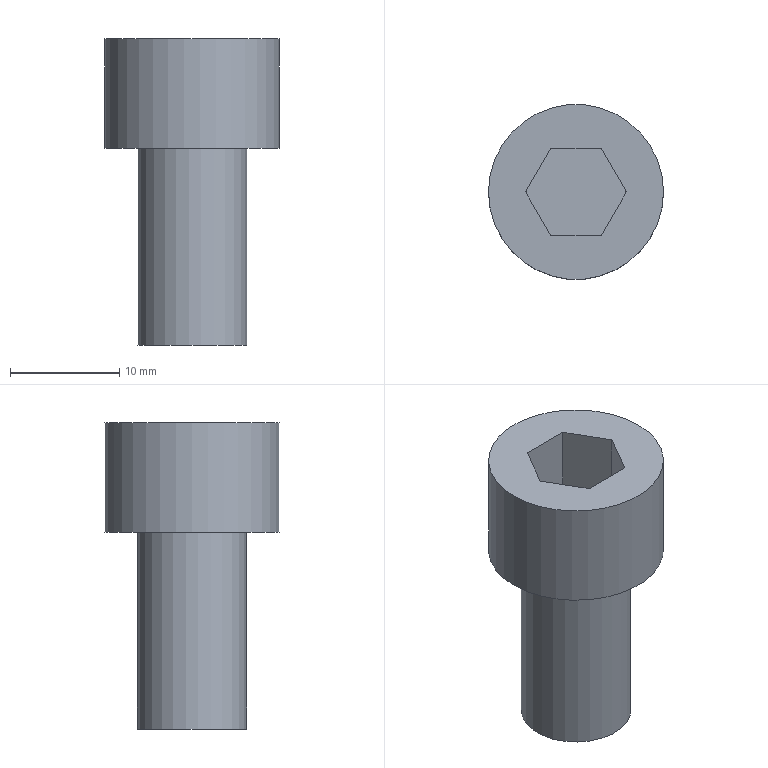Part | STEP file | 冲床-300配套压波_id138_x_t | 1 solid | 12 faces | box 16 x 16 x 28 mm | volume 3059 mm3 | plane 10 | cylinder 2 | commonest cylinder face diameters 10 x1 16 x1
STEP:
#1=CARTESIAN_POINT('',(1204.,86.,299.));
#2=VERTEX_POINT('',#1);
#3=CARTESIAN_POINT('',(1196.,86.,299.));
#4=DIRECTION('',(0.,0.,1.));
#5=DIRECTION('',(1.,0.,0.));
#6=AXIS2_PLACEMENT_3D('',#3,#4,#5);
#7=CIRCLE('',#6,8.);
#8=EDGE_CURVE('',#2,#2,#7,.T.);
#9=ORIENTED_EDGE('',*,*,#8,.T.);
#10=EDGE_LOOP('',(#9));
#11=FACE_BOUND('',#10,.T.);
#12=CARTESIAN_POINT('',(1193.691,90.,299.));
#13=VERTEX_POINT('',#12);
#14=CARTESIAN_POINT('',(1198.309,90.,299.));
#15=VERTEX_POINT('',#14);
#16=CARTESIAN_POINT('',(1193.691,90.,299.));
#17=DIRECTION('',(1.,0.,0.));
#18=VECTOR('',#17,1.);
#19=LINE('',#16,#18);
#20=EDGE_CURVE('',#13,#15,#19,.T.);
#21=ORIENTED_EDGE('',*,*,#20,.T.);
#22=CARTESIAN_POINT('',(1200.619,86.,299.));
#23=VERTEX_POINT('',#22);
#24=CARTESIAN_POINT('',(1198.309,90.,299.));
#25=DIRECTION('',(0.5,-0.866,0.));
#26=VECTOR('',#25,1.);
#27=LINE('',#24,#26);
#28=EDGE_CURVE('',#15,#23,#27,.T.);
#29=ORIENTED_EDGE('',*,*,#28,.T.);
#30=CARTESIAN_POINT('',(1198.309,82.,299.));
#31=VERTEX_POINT('',#30);
#32=CARTESIAN_POINT('',(1200.619,86.,299.));
#33=DIRECTION('',(-0.5,-0.866,0.));
#34=VECTOR('',#33,1.);
#35=LINE('',#32,#34);
#36=EDGE_CURVE('',#23,#31,#35,.T.);
#37=ORIENTED_EDGE('',*,*,#36,.T.);
#38=CARTESIAN_POINT('',(1193.691,82.,299.));
#39=VERTEX_POINT('',#38);
#40=CARTESIAN_POINT('',(1198.309,82.,299.));
#41=DIRECTION('',(-1.,0.,0.));
#42=VECTOR('',#41,1.);
#43=LINE('',#40,#42);
#44=EDGE_CURVE('',#31,#39,#43,.T.);
#45=ORIENTED_EDGE('',*,*,#44,.T.);
#46=CARTESIAN_POINT('',(1191.381,86.,299.));
#47=VERTEX_POINT('',#46);
#48=CARTESIAN_POINT('',(1193.691,82.,299.));
#49=DIRECTION('',(-0.5,0.866,0.));
#50=VECTOR('',#49,1.);
#51=LINE('',#48,#50);
#52=EDGE_CURVE('',#39,#47,#51,.T.);
#53=ORIENTED_EDGE('',*,*,#52,.T.);
#54=CARTESIAN_POINT('',(1191.381,86.,299.));
#55=DIRECTION('',(0.5,0.866,0.));
#56=VECTOR('',#55,1.);
#57=LINE('',#54,#56);
#58=EDGE_CURVE('',#47,#13,#57,.T.);
#59=ORIENTED_EDGE('',*,*,#58,.T.);
#60=EDGE_LOOP('',(#21,#29,#37,#45,#53,#59));
#61=FACE_BOUND('',#60,.T.);
#62=CARTESIAN_POINT('',(1204.,86.,299.));
#63=DIRECTION('',(0.,0.,-1.));
#64=DIRECTION('',(-1.,0.,0.));
#65=AXIS2_PLACEMENT_3D('',#62,#63,#64);
#66=PLANE('',#65);
#67=ADVANCED_FACE('',(#11,#61),#66,.F.);
#68=ORIENTED_EDGE('',*,*,#8,.F.);
#69=EDGE_LOOP('',(#68));
#70=FACE_BOUND('',#69,.T.);
#71=CARTESIAN_POINT('',(1204.,86.,289.));
#72=VERTEX_POINT('',#71);
#73=CARTESIAN_POINT('',(1196.,86.,289.));
#74=DIRECTION('',(0.,0.,1.));
#75=DIRECTION('',(1.,0.,0.));
#76=AXIS2_PLACEMENT_3D('',#73,#74,#75);
#77=CIRCLE('',#76,8.);
#78=EDGE_CURVE('',#72,#72,#77,.T.);
#79=ORIENTED_EDGE('',*,*,#78,.T.);
#80=EDGE_LOOP('',(#79));
#81=FACE_BOUND('',#80,.T.);
#82=CARTESIAN_POINT('',(1196.,86.,290.1));
#83=DIRECTION('',(0.,0.,1.));
#84=DIRECTION('',(1.,0.,0.));
#85=AXIS2_PLACEMENT_3D('',#82,#83,#84);
#86=CYLINDRICAL_SURFACE('',#85,8.);
#87=ADVANCED_FACE('',(#70,#81),#86,.T.);
#88=ORIENTED_EDGE('',*,*,#78,.F.);
#89=EDGE_LOOP('',(#88));
#90=FACE_BOUND('',#89,.T.);
#91=CARTESIAN_POINT('',(1201.,86.,289.));
#92=VERTEX_POINT('',#91);
#93=CARTESIAN_POINT('',(1196.,86.,289.));
#94=DIRECTION('',(0.,0.,1.));
#95=DIRECTION('',(1.,0.,0.));
#96=AXIS2_PLACEMENT_3D('',#93,#94,#95);
#97=CIRCLE('',#96,5.);
#98=EDGE_CURVE('',#92,#92,#97,.T.);
#99=ORIENTED_EDGE('',*,*,#98,.T.);
#100=EDGE_LOOP('',(#99));
#101=FACE_BOUND('',#100,.T.);
#102=CARTESIAN_POINT('',(1201.,86.,289.));
#103=DIRECTION('',(0.,0.,1.));
#104=DIRECTION('',(1.,0.,0.));
#105=AXIS2_PLACEMENT_3D('',#102,#103,#104);
#106=PLANE('',#105);
#107=ADVANCED_FACE('',(#90,#101),#106,.F.);
#108=ORIENTED_EDGE('',*,*,#98,.F.);
#109=EDGE_LOOP('',(#108));
#110=FACE_BOUND('',#109,.T.);
#111=CARTESIAN_POINT('',(1201.,86.,271.));
#112=VERTEX_POINT('',#111);
#113=CARTESIAN_POINT('',(1196.,86.,271.));
#114=DIRECTION('',(0.,0.,1.));
#115=DIRECTION('',(1.,0.,0.));
#116=AXIS2_PLACEMENT_3D('',#113,#114,#115);
#117=CIRCLE('',#116,5.);
#118=EDGE_CURVE('',#112,#112,#117,.T.);
#119=ORIENTED_EDGE('',*,*,#118,.T.);
#120=EDGE_LOOP('',(#119));
#121=FACE_BOUND('',#120,.T.);
#122=CARTESIAN_POINT('',(1196.,86.,290.1));
#123=DIRECTION('',(0.,0.,1.));
#124=DIRECTION('',(1.,0.,0.));
#125=AXIS2_PLACEMENT_3D('',#122,#123,#124);
#126=CYLINDRICAL_SURFACE('',#125,5.);
#127=ADVANCED_FACE('',(#110,#121),#126,.T.);
#128=ORIENTED_EDGE('',*,*,#118,.F.);
#129=EDGE_LOOP('',(#128));
#130=FACE_OUTER_BOUND('',#129,.T.);
#131=CARTESIAN_POINT('',(1196.,86.,271.));
#132=DIRECTION('',(0.,0.,1.));
#133=DIRECTION('',(1.,0.,0.));
#134=AXIS2_PLACEMENT_3D('',#131,#132,#133);
#135=PLANE('',#134);
#136=ADVANCED_FACE('',(#130),#135,.F.);
#137=ORIENTED_EDGE('',*,*,#20,.F.);
#138=CARTESIAN_POINT('',(1193.691,90.,292.4));
#139=VERTEX_POINT('',#138);
#140=CARTESIAN_POINT('',(1193.691,90.,292.4));
#141=DIRECTION('',(0.,0.,-1.));
#142=VECTOR('',#141,1.);
#143=LINE('',#140,#142);
#144=EDGE_CURVE('',#13,#139,#143,.T.);
#145=ORIENTED_EDGE('',*,*,#144,.T.);
#146=CARTESIAN_POINT('',(1198.309,90.,292.4));
#147=VERTEX_POINT('',#146);
#148=CARTESIAN_POINT('',(1193.691,90.,292.4));
#149=DIRECTION('',(-1.,0.,0.));
#150=VECTOR('',#149,1.);
#151=LINE('',#148,#150);
#152=EDGE_CURVE('',#147,#139,#151,.T.);
#153=ORIENTED_EDGE('',*,*,#152,.F.);
#154=CARTESIAN_POINT('',(1198.309,90.,292.4));
#155=DIRECTION('',(0.,0.,-1.));
#156=VECTOR('',#155,1.);
#157=LINE('',#154,#156);
#158=EDGE_CURVE('',#15,#147,#157,.T.);
#159=ORIENTED_EDGE('',*,*,#158,.F.);
#160=EDGE_LOOP('',(#137,#145,#153,#159));
#161=FACE_OUTER_BOUND('',#160,.T.);
#162=CARTESIAN_POINT('',(1193.691,90.,292.4));
#163=DIRECTION('',(0.,-1.,0.));
#164=DIRECTION('',(1.,0.,0.));
#165=AXIS2_PLACEMENT_3D('',#162,#163,#164);
#166=PLANE('',#165);
#167=ADVANCED_FACE('',(#161),#166,.T.);
#168=ORIENTED_EDGE('',*,*,#28,.F.);
#169=ORIENTED_EDGE('',*,*,#158,.T.);
#170=CARTESIAN_POINT('',(1200.619,86.,292.4));
#171=VERTEX_POINT('',#170);
#172=CARTESIAN_POINT('',(1198.309,90.,292.4));
#173=DIRECTION('',(-0.5,0.866,0.));
#174=VECTOR('',#173,1.);
#175=LINE('',#172,#174);
#176=EDGE_CURVE('',#171,#147,#175,.T.);
#177=ORIENTED_EDGE('',*,*,#176,.F.);
#178=CARTESIAN_POINT('',(1200.619,86.,292.4));
#179=DIRECTION('',(0.,0.,-1.));
#180=VECTOR('',#179,1.);
#181=LINE('',#178,#180);
#182=EDGE_CURVE('',#23,#171,#181,.T.);
#183=ORIENTED_EDGE('',*,*,#182,.F.);
#184=EDGE_LOOP('',(#168,#169,#177,#183));
#185=FACE_OUTER_BOUND('',#184,.T.);
#186=CARTESIAN_POINT('',(1198.309,90.,292.4));
#187=DIRECTION('',(-0.866,-0.5,0.));
#188=DIRECTION('',(0.5,-0.866,0.));
#189=AXIS2_PLACEMENT_3D('',#186,#187,#188);
#190=PLANE('',#189);
#191=ADVANCED_FACE('',(#185),#190,.T.);
#192=ORIENTED_EDGE('',*,*,#36,.F.);
#193=ORIENTED_EDGE('',*,*,#182,.T.);
#194=CARTESIAN_POINT('',(1198.309,82.,292.4));
#195=VERTEX_POINT('',#194);
#196=CARTESIAN_POINT('',(1200.619,86.,292.4));
#197=DIRECTION('',(0.5,0.866,0.));
#198=VECTOR('',#197,1.);
#199=LINE('',#196,#198);
#200=EDGE_CURVE('',#195,#171,#199,.T.);
#201=ORIENTED_EDGE('',*,*,#200,.F.);
#202=CARTESIAN_POINT('',(1198.309,82.,292.4));
#203=DIRECTION('',(0.,0.,-1.));
#204=VECTOR('',#203,1.);
#205=LINE('',#202,#204);
#206=EDGE_CURVE('',#31,#195,#205,.T.);
#207=ORIENTED_EDGE('',*,*,#206,.F.);
#208=EDGE_LOOP('',(#192,#193,#201,#207));
#209=FACE_OUTER_BOUND('',#208,.T.);
#210=CARTESIAN_POINT('',(1200.619,86.,292.4));
#211=DIRECTION('',(-0.866,0.5,0.));
#212=DIRECTION('',(-0.5,-0.866,0.));
#213=AXIS2_PLACEMENT_3D('',#210,#211,#212);
#214=PLANE('',#213);
#215=ADVANCED_FACE('',(#209),#214,.T.);
#216=ORIENTED_EDGE('',*,*,#44,.F.);
#217=ORIENTED_EDGE('',*,*,#206,.T.);
#218=CARTESIAN_POINT('',(1193.691,82.,292.4));
#219=VERTEX_POINT('',#218);
#220=CARTESIAN_POINT('',(1198.309,82.,292.4));
#221=DIRECTION('',(1.,0.,0.));
#222=VECTOR('',#221,1.);
#223=LINE('',#220,#222);
#224=EDGE_CURVE('',#219,#195,#223,.T.);
#225=ORIENTED_EDGE('',*,*,#224,.F.);
#226=CARTESIAN_POINT('',(1193.691,82.,292.4));
#227=DIRECTION('',(0.,0.,-1.));
#228=VECTOR('',#227,1.);
#229=LINE('',#226,#228);
#230=EDGE_CURVE('',#39,#219,#229,.T.);
#231=ORIENTED_EDGE('',*,*,#230,.F.);
#232=EDGE_LOOP('',(#216,#217,#225,#231));
#233=FACE_OUTER_BOUND('',#232,.T.);
#234=CARTESIAN_POINT('',(1198.309,82.,292.4));
#235=DIRECTION('',(0.,1.,0.));
#236=DIRECTION('',(0.,0.,1.));
#237=AXIS2_PLACEMENT_3D('',#234,#235,#236);
#238=PLANE('',#237);
#239=ADVANCED_FACE('',(#233),#238,.T.);
#240=ORIENTED_EDGE('',*,*,#52,.F.);
#241=ORIENTED_EDGE('',*,*,#230,.T.);
#242=CARTESIAN_POINT('',(1191.381,86.,292.4));
#243=VERTEX_POINT('',#242);
#244=CARTESIAN_POINT('',(1193.691,82.,292.4));
#245=DIRECTION('',(0.5,-0.866,0.));
#246=VECTOR('',#245,1.);
#247=LINE('',#244,#246);
#248=EDGE_CURVE('',#243,#219,#247,.T.);
#249=ORIENTED_EDGE('',*,*,#248,.F.);
#250=CARTESIAN_POINT('',(1191.381,86.,292.4));
#251=DIRECTION('',(0.,0.,-1.));
#252=VECTOR('',#251,1.);
#253=LINE('',#250,#252);
#254=EDGE_CURVE('',#47,#243,#253,.T.);
#255=ORIENTED_EDGE('',*,*,#254,.F.);
#256=EDGE_LOOP('',(#240,#241,#249,#255));
#257=FACE_OUTER_BOUND('',#256,.T.);
#258=CARTESIAN_POINT('',(1193.691,82.,292.4));
#259=DIRECTION('',(0.866,0.5,0.));
#260=DIRECTION('',(-0.5,0.866,0.));
#261=AXIS2_PLACEMENT_3D('',#258,#259,#260);
#262=PLANE('',#261);
#263=ADVANCED_FACE('',(#257),#262,.T.);
#264=ORIENTED_EDGE('',*,*,#58,.F.);
#265=ORIENTED_EDGE('',*,*,#254,.T.);
#266=CARTESIAN_POINT('',(1191.381,86.,292.4));
#267=DIRECTION('',(-0.5,-0.866,0.));
#268=VECTOR('',#267,1.);
#269=LINE('',#266,#268);
#270=EDGE_CURVE('',#139,#243,#269,.T.);
#271=ORIENTED_EDGE('',*,*,#270,.F.);
#272=ORIENTED_EDGE('',*,*,#144,.F.);
#273=EDGE_LOOP('',(#264,#265,#271,#272));
#274=FACE_OUTER_BOUND('',#273,.T.);
#275=CARTESIAN_POINT('',(1191.381,86.,292.4));
#276=DIRECTION('',(0.866,-0.5,0.));
#277=DIRECTION('',(0.5,0.866,0.));
#278=AXIS2_PLACEMENT_3D('',#275,#276,#277);
#279=PLANE('',#278);
#280=ADVANCED_FACE('',(#274),#279,.T.);
#281=ORIENTED_EDGE('',*,*,#152,.T.);
#282=ORIENTED_EDGE('',*,*,#270,.T.);
#283=ORIENTED_EDGE('',*,*,#248,.T.);
#284=ORIENTED_EDGE('',*,*,#224,.T.);
#285=ORIENTED_EDGE('',*,*,#200,.T.);
#286=ORIENTED_EDGE('',*,*,#176,.T.);
#287=EDGE_LOOP('',(#281,#282,#283,#284,#285,#286));
#288=FACE_OUTER_BOUND('',#287,.T.);
#289=CARTESIAN_POINT('',(1196.,86.,292.4));
#290=DIRECTION('',(0.,0.,-1.));
#291=DIRECTION('',(-1.,0.,0.));
#292=AXIS2_PLACEMENT_3D('',#289,#290,#291);
#293=PLANE('',#292);
#294=ADVANCED_FACE('',(#288),#293,.F.);
#295=CLOSED_SHELL('',(#67,#87,#107,#127,#136,#167,#191,#215,#239,#263,#280,#294));
#296=MANIFOLD_SOLID_BREP('',#295);
#297=(LENGTH_UNIT()NAMED_UNIT(*)SI_UNIT(.MILLI.,.METRE.));
#298=UNCERTAINTY_MEASURE_WITH_UNIT(LENGTH_MEASURE(0.00002),#297,'','');
#299=(NAMED_UNIT(*)PLANE_ANGLE_UNIT()SI_UNIT($,.RADIAN.));
#300=PLANE_ANGLE_MEASURE_WITH_UNIT(PLANE_ANGLE_MEASURE(0.01745),#299);
#301=DIMENSIONAL_EXPONENTS(0.,0.,0.,0.,0.,0.,0.);
#302=(CONVERSION_BASED_UNIT('DEGREE',#300)NAMED_UNIT(#301)PLANE_ANGLE_UNIT());
#303=(NAMED_UNIT(*)SI_UNIT($,.STERADIAN.)SOLID_ANGLE_UNIT());
#304=(GEOMETRIC_REPRESENTATION_CONTEXT(3)GLOBAL_UNCERTAINTY_ASSIGNED_CONTEXT((#298))GLOBAL_UNIT_ASSIGNED_CONTEXT((#297,#302,#303))REPRESENTATION_CONTEXT('',''));
#305=ADVANCED_BREP_SHAPE_REPRESENTATION('',(#296),#304);